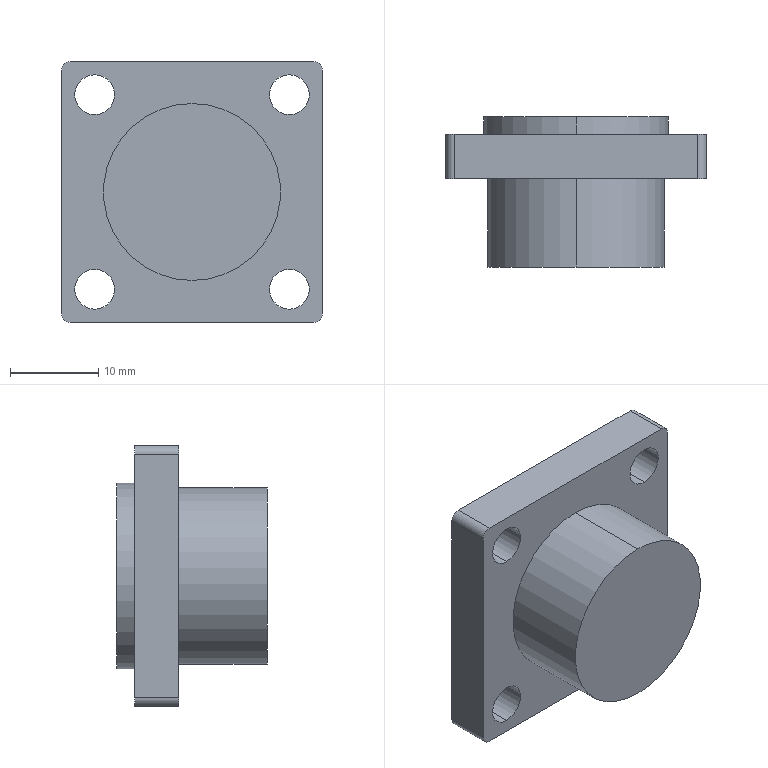Part | SolidWorks | features ICE 5, Extrusion 1, Fillet 1 | 1 solid | 29 faces | box 29.5 x 17 x 29.5 mm | volume 7218 mm3 | cylinder 16 | plane 13 | commonest cylinder face diameters 4.5 x8 2 x4 20 x2 21 x2
STEP:
#1=CARTESIAN_POINT('',(11.,10.,8.75));
#2=VERTEX_POINT('',#1);
#3=CARTESIAN_POINT('',(11.,10.,13.25));
#4=VERTEX_POINT('',#3);
#5=CARTESIAN_POINT('',(11.,10.,11.));
#6=DIRECTION('',(0.,1.,0.));
#7=DIRECTION('',(0.,0.,1.));
#8=AXIS2_PLACEMENT_3D('',#5,#6,#7);
#9=CIRCLE('',#8,2.25);
#10=EDGE_CURVE('',#2,#4,#9,.T.);
#11=ORIENTED_EDGE('',*,*,#10,.F.);
#12=CARTESIAN_POINT('',(11.,15.,8.75));
#13=VERTEX_POINT('',#12);
#14=CARTESIAN_POINT('',(11.,-2.,8.75));
#15=DIRECTION('',(0.,1.,0.));
#16=VECTOR('',#15,1000.);
#17=LINE('',#14,#16);
#18=EDGE_CURVE('',#2,#13,#17,.T.);
#19=ORIENTED_EDGE('',*,*,#18,.T.);
#20=CARTESIAN_POINT('',(11.,15.,13.25));
#21=VERTEX_POINT('',#20);
#22=CARTESIAN_POINT('',(11.,15.,11.));
#23=DIRECTION('',(0.,1.,0.));
#24=DIRECTION('',(0.,0.,1.));
#25=AXIS2_PLACEMENT_3D('',#22,#23,#24);
#26=CIRCLE('',#25,2.25);
#27=EDGE_CURVE('',#13,#21,#26,.T.);
#28=ORIENTED_EDGE('',*,*,#27,.T.);
#29=CARTESIAN_POINT('',(11.,-2.,13.25));
#30=DIRECTION('',(0.,1.,0.));
#31=VECTOR('',#30,1000.);
#32=LINE('',#29,#31);
#33=EDGE_CURVE('',#4,#21,#32,.T.);
#34=ORIENTED_EDGE('',*,*,#33,.F.);
#35=EDGE_LOOP('',(#11,#19,#28,#34));
#36=FACE_OUTER_BOUND('',#35,.T.);
#37=CARTESIAN_POINT('',(11.,-2.,11.));
#38=DIRECTION('',(0.,1.,0.));
#39=DIRECTION('',(0.,0.,1.));
#40=AXIS2_PLACEMENT_3D('',#37,#38,#39);
#41=CYLINDRICAL_SURFACE('',#40,2.25);
#42=ADVANCED_FACE('',(#36),#41,.F.);
#43=CARTESIAN_POINT('',(-11.,10.,8.75));
#44=VERTEX_POINT('',#43);
#45=CARTESIAN_POINT('',(-11.,10.,13.25));
#46=VERTEX_POINT('',#45);
#47=CARTESIAN_POINT('',(-11.,10.,11.));
#48=DIRECTION('',(0.,1.,0.));
#49=DIRECTION('',(0.,0.,1.));
#50=AXIS2_PLACEMENT_3D('',#47,#48,#49);
#51=CIRCLE('',#50,2.25);
#52=EDGE_CURVE('',#44,#46,#51,.T.);
#53=ORIENTED_EDGE('',*,*,#52,.F.);
#54=CARTESIAN_POINT('',(-11.,15.,8.75));
#55=VERTEX_POINT('',#54);
#56=CARTESIAN_POINT('',(-11.,-2.,8.75));
#57=DIRECTION('',(0.,1.,0.));
#58=VECTOR('',#57,1000.);
#59=LINE('',#56,#58);
#60=EDGE_CURVE('',#44,#55,#59,.T.);
#61=ORIENTED_EDGE('',*,*,#60,.T.);
#62=CARTESIAN_POINT('',(-11.,15.,13.25));
#63=VERTEX_POINT('',#62);
#64=CARTESIAN_POINT('',(-11.,15.,11.));
#65=DIRECTION('',(0.,1.,0.));
#66=DIRECTION('',(0.,0.,1.));
#67=AXIS2_PLACEMENT_3D('',#64,#65,#66);
#68=CIRCLE('',#67,2.25);
#69=EDGE_CURVE('',#55,#63,#68,.T.);
#70=ORIENTED_EDGE('',*,*,#69,.T.);
#71=CARTESIAN_POINT('',(-11.,-2.,13.25));
#72=DIRECTION('',(0.,1.,0.));
#73=VECTOR('',#72,1000.);
#74=LINE('',#71,#73);
#75=EDGE_CURVE('',#46,#63,#74,.T.);
#76=ORIENTED_EDGE('',*,*,#75,.F.);
#77=EDGE_LOOP('',(#53,#61,#70,#76));
#78=FACE_OUTER_BOUND('',#77,.T.);
#79=CARTESIAN_POINT('',(-11.,-2.,11.));
#80=DIRECTION('',(0.,1.,0.));
#81=DIRECTION('',(0.,0.,1.));
#82=AXIS2_PLACEMENT_3D('',#79,#80,#81);
#83=CYLINDRICAL_SURFACE('',#82,2.25);
#84=ADVANCED_FACE('',(#78),#83,.F.);
#85=CARTESIAN_POINT('',(-11.,10.,-13.25));
#86=VERTEX_POINT('',#85);
#87=CARTESIAN_POINT('',(-11.,10.,-8.75));
#88=VERTEX_POINT('',#87);
#89=CARTESIAN_POINT('',(-11.,10.,-11.));
#90=DIRECTION('',(0.,1.,0.));
#91=DIRECTION('',(0.,0.,1.));
#92=AXIS2_PLACEMENT_3D('',#89,#90,#91);
#93=CIRCLE('',#92,2.25);
#94=EDGE_CURVE('',#86,#88,#93,.T.);
#95=ORIENTED_EDGE('',*,*,#94,.F.);
#96=CARTESIAN_POINT('',(-11.,15.,-13.25));
#97=VERTEX_POINT('',#96);
#98=CARTESIAN_POINT('',(-11.,-2.,-13.25));
#99=DIRECTION('',(0.,1.,0.));
#100=VECTOR('',#99,1000.);
#101=LINE('',#98,#100);
#102=EDGE_CURVE('',#86,#97,#101,.T.);
#103=ORIENTED_EDGE('',*,*,#102,.T.);
#104=CARTESIAN_POINT('',(-11.,15.,-8.75));
#105=VERTEX_POINT('',#104);
#106=CARTESIAN_POINT('',(-11.,15.,-11.));
#107=DIRECTION('',(0.,1.,0.));
#108=DIRECTION('',(0.,0.,1.));
#109=AXIS2_PLACEMENT_3D('',#106,#107,#108);
#110=CIRCLE('',#109,2.25);
#111=EDGE_CURVE('',#97,#105,#110,.T.);
#112=ORIENTED_EDGE('',*,*,#111,.T.);
#113=CARTESIAN_POINT('',(-11.,-2.,-8.75));
#114=DIRECTION('',(0.,1.,0.));
#115=VECTOR('',#114,1000.);
#116=LINE('',#113,#115);
#117=EDGE_CURVE('',#88,#105,#116,.T.);
#118=ORIENTED_EDGE('',*,*,#117,.F.);
#119=EDGE_LOOP('',(#95,#103,#112,#118));
#120=FACE_OUTER_BOUND('',#119,.T.);
#121=CARTESIAN_POINT('',(-11.,-2.,-11.));
#122=DIRECTION('',(0.,1.,0.));
#123=DIRECTION('',(0.,0.,1.));
#124=AXIS2_PLACEMENT_3D('',#121,#122,#123);
#125=CYLINDRICAL_SURFACE('',#124,2.25);
#126=ADVANCED_FACE('',(#120),#125,.F.);
#127=CARTESIAN_POINT('',(11.,10.,-13.25));
#128=VERTEX_POINT('',#127);
#129=CARTESIAN_POINT('',(11.,10.,-8.75));
#130=VERTEX_POINT('',#129);
#131=CARTESIAN_POINT('',(11.,10.,-11.));
#132=DIRECTION('',(0.,1.,0.));
#133=DIRECTION('',(0.,0.,1.));
#134=AXIS2_PLACEMENT_3D('',#131,#132,#133);
#135=CIRCLE('',#134,2.25);
#136=EDGE_CURVE('',#128,#130,#135,.T.);
#137=ORIENTED_EDGE('',*,*,#136,.F.);
#138=CARTESIAN_POINT('',(11.,15.,-13.25));
#139=VERTEX_POINT('',#138);
#140=CARTESIAN_POINT('',(11.,-2.,-13.25));
#141=DIRECTION('',(0.,1.,0.));
#142=VECTOR('',#141,1000.);
#143=LINE('',#140,#142);
#144=EDGE_CURVE('',#128,#139,#143,.T.);
#145=ORIENTED_EDGE('',*,*,#144,.T.);
#146=CARTESIAN_POINT('',(11.,15.,-8.75));
#147=VERTEX_POINT('',#146);
#148=CARTESIAN_POINT('',(11.,15.,-11.));
#149=DIRECTION('',(0.,1.,0.));
#150=DIRECTION('',(0.,0.,1.));
#151=AXIS2_PLACEMENT_3D('',#148,#149,#150);
#152=CIRCLE('',#151,2.25);
#153=EDGE_CURVE('',#139,#147,#152,.T.);
#154=ORIENTED_EDGE('',*,*,#153,.T.);
#155=CARTESIAN_POINT('',(11.,-2.,-8.75));
#156=DIRECTION('',(0.,1.,0.));
#157=VECTOR('',#156,1000.);
#158=LINE('',#155,#157);
#159=EDGE_CURVE('',#130,#147,#158,.T.);
#160=ORIENTED_EDGE('',*,*,#159,.F.);
#161=EDGE_LOOP('',(#137,#145,#154,#160));
#162=FACE_OUTER_BOUND('',#161,.T.);
#163=CARTESIAN_POINT('',(11.,-2.,-11.));
#164=DIRECTION('',(0.,1.,0.));
#165=DIRECTION('',(0.,0.,1.));
#166=AXIS2_PLACEMENT_3D('',#163,#164,#165);
#167=CYLINDRICAL_SURFACE('',#166,2.25);
#168=ADVANCED_FACE('',(#162),#167,.F.);
#169=CARTESIAN_POINT('',(0.,10.,10.));
#170=VERTEX_POINT('',#169);
#171=CARTESIAN_POINT('',(0.,10.,-10.));
#172=VERTEX_POINT('',#171);
#173=CARTESIAN_POINT('',(0.,10.,0.));
#174=DIRECTION('',(0.,1.,0.));
#175=DIRECTION('',(0.,0.,1.));
#176=AXIS2_PLACEMENT_3D('',#173,#174,#175);
#177=CIRCLE('',#176,10.);
#178=EDGE_CURVE('',#170,#172,#177,.T.);
#179=ORIENTED_EDGE('',*,*,#178,.F.);
#180=CARTESIAN_POINT('',(0.,0.,10.));
#181=VERTEX_POINT('',#180);
#182=CARTESIAN_POINT('',(0.,10.,10.));
#183=DIRECTION('',(0.,-1.,0.));
#184=VECTOR('',#183,1000.);
#185=LINE('',#182,#184);
#186=EDGE_CURVE('',#170,#181,#185,.T.);
#187=ORIENTED_EDGE('',*,*,#186,.T.);
#188=CARTESIAN_POINT('',(0.,0.,-10.));
#189=VERTEX_POINT('',#188);
#190=CARTESIAN_POINT('',(0.,0.,0.));
#191=DIRECTION('',(0.,1.,0.));
#192=DIRECTION('',(0.,0.,1.));
#193=AXIS2_PLACEMENT_3D('',#190,#191,#192);
#194=CIRCLE('',#193,10.);
#195=EDGE_CURVE('',#181,#189,#194,.T.);
#196=ORIENTED_EDGE('',*,*,#195,.T.);
#197=CARTESIAN_POINT('',(0.,10.,-10.));
#198=DIRECTION('',(0.,-1.,0.));
#199=VECTOR('',#198,1000.);
#200=LINE('',#197,#199);
#201=EDGE_CURVE('',#172,#189,#200,.T.);
#202=ORIENTED_EDGE('',*,*,#201,.F.);
#203=EDGE_LOOP('',(#179,#187,#196,#202));
#204=FACE_OUTER_BOUND('',#203,.T.);
#205=CARTESIAN_POINT('',(0.,10.,0.));
#206=DIRECTION('',(0.,-1.,0.));
#207=DIRECTION('',(0.,0.,-1.));
#208=AXIS2_PLACEMENT_3D('',#205,#206,#207);
#209=CYLINDRICAL_SURFACE('',#208,10.);
#210=ADVANCED_FACE('',(#204),#209,.T.);
#211=CARTESIAN_POINT('',(0.,17.,10.5));
#212=VERTEX_POINT('',#211);
#213=CARTESIAN_POINT('',(0.,17.,-10.5));
#214=VERTEX_POINT('',#213);
#215=CARTESIAN_POINT('',(0.,17.,0.));
#216=DIRECTION('',(0.,1.,0.));
#217=DIRECTION('',(0.,0.,1.));
#218=AXIS2_PLACEMENT_3D('',#215,#216,#217);
#219=CIRCLE('',#218,10.5);
#220=EDGE_CURVE('',#212,#214,#219,.T.);
#221=ORIENTED_EDGE('',*,*,#220,.F.);
#222=CARTESIAN_POINT('',(0.,15.,10.5));
#223=VERTEX_POINT('',#222);
#224=CARTESIAN_POINT('',(0.,32.,10.5));
#225=DIRECTION('',(0.,-1.,0.));
#226=VECTOR('',#225,1000.);
#227=LINE('',#224,#226);
#228=EDGE_CURVE('',#212,#223,#227,.T.);
#229=ORIENTED_EDGE('',*,*,#228,.T.);
#230=CARTESIAN_POINT('',(0.,15.,-10.5));
#231=VERTEX_POINT('',#230);
#232=CARTESIAN_POINT('',(0.,15.,0.));
#233=DIRECTION('',(0.,1.,0.));
#234=DIRECTION('',(0.,0.,1.));
#235=AXIS2_PLACEMENT_3D('',#232,#233,#234);
#236=CIRCLE('',#235,10.5);
#237=EDGE_CURVE('',#223,#231,#236,.T.);
#238=ORIENTED_EDGE('',*,*,#237,.T.);
#239=CARTESIAN_POINT('',(0.,32.,-10.5));
#240=DIRECTION('',(0.,-1.,0.));
#241=VECTOR('',#240,1000.);
#242=LINE('',#239,#241);
#243=EDGE_CURVE('',#214,#231,#242,.T.);
#244=ORIENTED_EDGE('',*,*,#243,.F.);
#245=EDGE_LOOP('',(#221,#229,#238,#244));
#246=FACE_OUTER_BOUND('',#245,.T.);
#247=CARTESIAN_POINT('',(0.,32.,0.));
#248=DIRECTION('',(0.,-1.,0.));
#249=DIRECTION('',(0.,0.,-1.));
#250=AXIS2_PLACEMENT_3D('',#247,#248,#249);
#251=CYLINDRICAL_SURFACE('',#250,10.5);
#252=ADVANCED_FACE('',(#246),#251,.T.);
#253=ORIENTED_EDGE('',*,*,#228,.F.);
#254=CARTESIAN_POINT('',(0.,17.,0.));
#255=DIRECTION('',(0.,1.,0.));
#256=DIRECTION('',(0.,0.,1.));
#257=AXIS2_PLACEMENT_3D('',#254,#255,#256);
#258=CIRCLE('',#257,10.5);
#259=EDGE_CURVE('',#214,#212,#258,.T.);
#260=ORIENTED_EDGE('',*,*,#259,.F.);
#261=ORIENTED_EDGE('',*,*,#243,.T.);
#262=CARTESIAN_POINT('',(0.,15.,0.));
#263=DIRECTION('',(0.,1.,0.));
#264=DIRECTION('',(0.,0.,1.));
#265=AXIS2_PLACEMENT_3D('',#262,#263,#264);
#266=CIRCLE('',#265,10.5);
#267=EDGE_CURVE('',#231,#223,#266,.T.);
#268=ORIENTED_EDGE('',*,*,#267,.T.);
#269=EDGE_LOOP('',(#253,#260,#261,#268));
#270=FACE_OUTER_BOUND('',#269,.T.);
#271=CARTESIAN_POINT('',(0.,32.,0.));
#272=DIRECTION('',(0.,-1.,0.));
#273=DIRECTION('',(0.,0.,-1.));
#274=AXIS2_PLACEMENT_3D('',#271,#272,#273);
#275=CYLINDRICAL_SURFACE('',#274,10.5);
#276=ADVANCED_FACE('',(#270),#275,.T.);
#277=CARTESIAN_POINT('',(11.,15.,11.));
#278=DIRECTION('',(0.,1.,0.));
#279=DIRECTION('',(0.,0.,1.));
#280=AXIS2_PLACEMENT_3D('',#277,#278,#279);
#281=CIRCLE('',#280,2.25);
#282=EDGE_CURVE('',#21,#13,#281,.T.);
#283=ORIENTED_EDGE('',*,*,#282,.F.);
#284=ORIENTED_EDGE('',*,*,#27,.F.);
#285=EDGE_LOOP('',(#283,#284));
#286=FACE_BOUND('',#285,.T.);
#287=CARTESIAN_POINT('',(-11.,15.,11.));
#288=DIRECTION('',(0.,1.,0.));
#289=DIRECTION('',(0.,0.,1.));
#290=AXIS2_PLACEMENT_3D('',#287,#288,#289);
#291=CIRCLE('',#290,2.25);
#292=EDGE_CURVE('',#63,#55,#291,.T.);
#293=ORIENTED_EDGE('',*,*,#292,.F.);
#294=ORIENTED_EDGE('',*,*,#69,.F.);
#295=EDGE_LOOP('',(#293,#294));
#296=FACE_BOUND('',#295,.T.);
#297=CARTESIAN_POINT('',(-11.,15.,-11.));
#298=DIRECTION('',(0.,1.,0.));
#299=DIRECTION('',(0.,0.,1.));
#300=AXIS2_PLACEMENT_3D('',#297,#298,#299);
#301=CIRCLE('',#300,2.25);
#302=EDGE_CURVE('',#105,#97,#301,.T.);
#303=ORIENTED_EDGE('',*,*,#302,.F.);
#304=ORIENTED_EDGE('',*,*,#111,.F.);
#305=EDGE_LOOP('',(#303,#304));
#306=FACE_BOUND('',#305,.T.);
#307=CARTESIAN_POINT('',(11.,15.,-11.));
#308=DIRECTION('',(0.,1.,0.));
#309=DIRECTION('',(0.,0.,1.));
#310=AXIS2_PLACEMENT_3D('',#307,#308,#309);
#311=CIRCLE('',#310,2.25);
#312=EDGE_CURVE('',#147,#139,#311,.T.);
#313=ORIENTED_EDGE('',*,*,#312,.F.);
#314=ORIENTED_EDGE('',*,*,#153,.F.);
#315=EDGE_LOOP('',(#313,#314));
#316=FACE_BOUND('',#315,.T.);
#317=CARTESIAN_POINT('',(13.75,15.,-14.75));
#318=VERTEX_POINT('',#317);
#319=CARTESIAN_POINT('',(-13.75,15.,-14.75));
#320=VERTEX_POINT('',#319);
#321=CARTESIAN_POINT('',(-14.75,15.,-14.75));
#322=DIRECTION('',(-1.,0.,0.));
#323=VECTOR('',#322,1000.);
#324=LINE('',#321,#323);
#325=EDGE_CURVE('',#318,#320,#324,.T.);
#326=ORIENTED_EDGE('',*,*,#325,.T.);
#327=CARTESIAN_POINT('',(-14.75,15.,-13.75));
#328=VERTEX_POINT('',#327);
#329=CARTESIAN_POINT('',(-13.75,15.,-13.75));
#330=DIRECTION('',(0.,1.,0.));
#331=DIRECTION('',(0.,0.,1.));
#332=AXIS2_PLACEMENT_3D('',#329,#330,#331);
#333=CIRCLE('',#332,1.);
#334=EDGE_CURVE('',#320,#328,#333,.T.);
#335=ORIENTED_EDGE('',*,*,#334,.T.);
#336=CARTESIAN_POINT('',(-14.75,15.,13.75));
#337=VERTEX_POINT('',#336);
#338=CARTESIAN_POINT('',(-14.75,15.,-14.75));
#339=DIRECTION('',(0.,0.,1.));
#340=VECTOR('',#339,1000.);
#341=LINE('',#338,#340);
#342=EDGE_CURVE('',#328,#337,#341,.T.);
#343=ORIENTED_EDGE('',*,*,#342,.T.);
#344=CARTESIAN_POINT('',(-13.75,15.,14.75));
#345=VERTEX_POINT('',#344);
#346=CARTESIAN_POINT('',(-13.75,15.,13.75));
#347=DIRECTION('',(0.,1.,0.));
#348=DIRECTION('',(0.,0.,1.));
#349=AXIS2_PLACEMENT_3D('',#346,#347,#348);
#350=CIRCLE('',#349,1.);
#351=EDGE_CURVE('',#337,#345,#350,.T.);
#352=ORIENTED_EDGE('',*,*,#351,.T.);
#353=CARTESIAN_POINT('',(13.75,15.,14.75));
#354=VERTEX_POINT('',#353);
#355=CARTESIAN_POINT('',(-14.75,15.,14.75));
#356=DIRECTION('',(1.,0.,0.));
#357=VECTOR('',#356,1000.);
#358=LINE('',#355,#357);
#359=EDGE_CURVE('',#345,#354,#358,.T.);
#360=ORIENTED_EDGE('',*,*,#359,.T.);
#361=CARTESIAN_POINT('',(14.75,15.,13.75));
#362=VERTEX_POINT('',#361);
#363=CARTESIAN_POINT('',(13.75,15.,13.75));
#364=DIRECTION('',(0.,1.,0.));
#365=DIRECTION('',(0.,0.,1.));
#366=AXIS2_PLACEMENT_3D('',#363,#364,#365);
#367=CIRCLE('',#366,1.);
#368=EDGE_CURVE('',#354,#362,#367,.T.);
#369=ORIENTED_EDGE('',*,*,#368,.T.);
#370=CARTESIAN_POINT('',(14.75,15.,-13.75));
#371=VERTEX_POINT('',#370);
#372=CARTESIAN_POINT('',(14.75,15.,-14.75));
#373=DIRECTION('',(0.,0.,-1.));
#374=VECTOR('',#373,1000.);
#375=LINE('',#372,#374);
#376=EDGE_CURVE('',#362,#371,#375,.T.);
#377=ORIENTED_EDGE('',*,*,#376,.T.);
#378=CARTESIAN_POINT('',(13.75,15.,-13.75));
#379=DIRECTION('',(0.,1.,0.));
#380=DIRECTION('',(0.,0.,1.));
#381=AXIS2_PLACEMENT_3D('',#378,#379,#380);
#382=CIRCLE('',#381,1.);
#383=EDGE_CURVE('',#371,#318,#382,.T.);
#384=ORIENTED_EDGE('',*,*,#383,.T.);
#385=EDGE_LOOP('',(#326,#335,#343,#352,#360,#369,#377,#384));
#386=FACE_OUTER_BOUND('',#385,.T.);
#387=ORIENTED_EDGE('',*,*,#267,.F.);
#388=ORIENTED_EDGE('',*,*,#237,.F.);
#389=EDGE_LOOP('',(#387,#388));
#390=FACE_BOUND('',#389,.T.);
#391=CARTESIAN_POINT('',(0.,15.,0.));
#392=DIRECTION('',(0.,1.,0.));
#393=DIRECTION('',(0.,0.,1.));
#394=AXIS2_PLACEMENT_3D('',#391,#392,#393);
#395=PLANE('',#394);
#396=ADVANCED_FACE('',(#286,#296,#306,#316,#386,#390),#395,.T.);
#397=ORIENTED_EDGE('',*,*,#186,.F.);
#398=CARTESIAN_POINT('',(0.,10.,0.));
#399=DIRECTION('',(0.,1.,0.));
#400=DIRECTION('',(0.,0.,1.));
#401=AXIS2_PLACEMENT_3D('',#398,#399,#400);
#402=CIRCLE('',#401,10.);
#403=EDGE_CURVE('',#172,#170,#402,.T.);
#404=ORIENTED_EDGE('',*,*,#403,.F.);
#405=ORIENTED_EDGE('',*,*,#201,.T.);
#406=CARTESIAN_POINT('',(0.,0.,0.));
#407=DIRECTION('',(0.,1.,0.));
#408=DIRECTION('',(0.,0.,1.));
#409=AXIS2_PLACEMENT_3D('',#406,#407,#408);
#410=CIRCLE('',#409,10.);
#411=EDGE_CURVE('',#189,#181,#410,.T.);
#412=ORIENTED_EDGE('',*,*,#411,.T.);
#413=EDGE_LOOP('',(#397,#404,#405,#412));
#414=FACE_OUTER_BOUND('',#413,.T.);
#415=CARTESIAN_POINT('',(0.,10.,0.));
#416=DIRECTION('',(0.,-1.,0.));
#417=DIRECTION('',(0.,0.,-1.));
#418=AXIS2_PLACEMENT_3D('',#415,#416,#417);
#419=CYLINDRICAL_SURFACE('',#418,10.);
#420=ADVANCED_FACE('',(#414),#419,.T.);
#421=ORIENTED_EDGE('',*,*,#411,.F.);
#422=ORIENTED_EDGE('',*,*,#195,.F.);
#423=EDGE_LOOP('',(#421,#422));
#424=FACE_OUTER_BOUND('',#423,.T.);
#425=CARTESIAN_POINT('',(0.,0.,0.));
#426=DIRECTION('',(0.,1.,0.));
#427=DIRECTION('',(0.,0.,1.));
#428=AXIS2_PLACEMENT_3D('',#425,#426,#427);
#429=PLANE('',#428);
#430=ADVANCED_FACE('',(#424),#429,.F.);
#431=CARTESIAN_POINT('',(11.,10.,11.));
#432=DIRECTION('',(0.,1.,0.));
#433=DIRECTION('',(0.,0.,1.));
#434=AXIS2_PLACEMENT_3D('',#431,#432,#433);
#435=CIRCLE('',#434,2.25);
#436=EDGE_CURVE('',#4,#2,#435,.T.);
#437=ORIENTED_EDGE('',*,*,#436,.T.);
#438=ORIENTED_EDGE('',*,*,#10,.T.);
#439=EDGE_LOOP('',(#437,#438));
#440=FACE_BOUND('',#439,.T.);
#441=CARTESIAN_POINT('',(-11.,10.,11.));
#442=DIRECTION('',(0.,1.,0.));
#443=DIRECTION('',(0.,0.,1.));
#444=AXIS2_PLACEMENT_3D('',#441,#442,#443);
#445=CIRCLE('',#444,2.25);
#446=EDGE_CURVE('',#46,#44,#445,.T.);
#447=ORIENTED_EDGE('',*,*,#446,.T.);
#448=ORIENTED_EDGE('',*,*,#52,.T.);
#449=EDGE_LOOP('',(#447,#448));
#450=FACE_BOUND('',#449,.T.);
#451=CARTESIAN_POINT('',(-11.,10.,-11.));
#452=DIRECTION('',(0.,1.,0.));
#453=DIRECTION('',(0.,0.,1.));
#454=AXIS2_PLACEMENT_3D('',#451,#452,#453);
#455=CIRCLE('',#454,2.25);
#456=EDGE_CURVE('',#88,#86,#455,.T.);
#457=ORIENTED_EDGE('',*,*,#456,.T.);
#458=ORIENTED_EDGE('',*,*,#94,.T.);
#459=EDGE_LOOP('',(#457,#458));
#460=FACE_BOUND('',#459,.T.);
#461=CARTESIAN_POINT('',(11.,10.,-11.));
#462=DIRECTION('',(0.,1.,0.));
#463=DIRECTION('',(0.,0.,1.));
#464=AXIS2_PLACEMENT_3D('',#461,#462,#463);
#465=CIRCLE('',#464,2.25);
#466=EDGE_CURVE('',#130,#128,#465,.T.);
#467=ORIENTED_EDGE('',*,*,#466,.T.);
#468=ORIENTED_EDGE('',*,*,#136,.T.);
#469=EDGE_LOOP('',(#467,#468));
#470=FACE_BOUND('',#469,.T.);
#471=CARTESIAN_POINT('',(-14.75,10.,-13.75));
#472=VERTEX_POINT('',#471);
#473=CARTESIAN_POINT('',(-14.75,10.,13.75));
#474=VERTEX_POINT('',#473);
#475=CARTESIAN_POINT('',(-14.75,10.,-14.75));
#476=DIRECTION('',(0.,0.,1.));
#477=VECTOR('',#476,1000.);
#478=LINE('',#475,#477);
#479=EDGE_CURVE('',#472,#474,#478,.T.);
#480=ORIENTED_EDGE('',*,*,#479,.F.);
#481=CARTESIAN_POINT('',(-13.75,10.,-14.75));
#482=VERTEX_POINT('',#481);
#483=CARTESIAN_POINT('',(-13.75,10.,-13.75));
#484=DIRECTION('',(0.,-1.,0.));
#485=DIRECTION('',(0.,0.,1.));
#486=AXIS2_PLACEMENT_3D('',#483,#484,#485);
#487=CIRCLE('',#486,1.);
#488=EDGE_CURVE('',#472,#482,#487,.T.);
#489=ORIENTED_EDGE('',*,*,#488,.T.);
#490=CARTESIAN_POINT('',(13.75,10.,-14.75));
#491=VERTEX_POINT('',#490);
#492=CARTESIAN_POINT('',(-14.75,10.,-14.75));
#493=DIRECTION('',(-1.,0.,0.));
#494=VECTOR('',#493,1000.);
#495=LINE('',#492,#494);
#496=EDGE_CURVE('',#491,#482,#495,.T.);
#497=ORIENTED_EDGE('',*,*,#496,.F.);
#498=CARTESIAN_POINT('',(14.75,10.,-13.75));
#499=VERTEX_POINT('',#498);
#500=CARTESIAN_POINT('',(13.75,10.,-13.75));
#501=DIRECTION('',(0.,-1.,0.));
#502=DIRECTION('',(0.,0.,1.));
#503=AXIS2_PLACEMENT_3D('',#500,#501,#502);
#504=CIRCLE('',#503,1.);
#505=EDGE_CURVE('',#491,#499,#504,.T.);
#506=ORIENTED_EDGE('',*,*,#505,.T.);
#507=CARTESIAN_POINT('',(14.75,10.,13.75));
#508=VERTEX_POINT('',#507);
#509=CARTESIAN_POINT('',(14.75,10.,-14.75));
#510=DIRECTION('',(0.,0.,-1.));
#511=VECTOR('',#510,1000.);
#512=LINE('',#509,#511);
#513=EDGE_CURVE('',#508,#499,#512,.T.);
#514=ORIENTED_EDGE('',*,*,#513,.F.);
#515=CARTESIAN_POINT('',(13.75,10.,14.75));
#516=VERTEX_POINT('',#515);
#517=CARTESIAN_POINT('',(13.75,10.,13.75));
#518=DIRECTION('',(0.,-1.,0.));
#519=DIRECTION('',(0.,0.,1.));
#520=AXIS2_PLACEMENT_3D('',#517,#518,#519);
#521=CIRCLE('',#520,1.);
#522=EDGE_CURVE('',#508,#516,#521,.T.);
#523=ORIENTED_EDGE('',*,*,#522,.T.);
#524=CARTESIAN_POINT('',(-13.75,10.,14.75));
#525=VERTEX_POINT('',#524);
#526=CARTESIAN_POINT('',(-14.75,10.,14.75));
#527=DIRECTION('',(1.,0.,0.));
#528=VECTOR('',#527,1000.);
#529=LINE('',#526,#528);
#530=EDGE_CURVE('',#525,#516,#529,.T.);
#531=ORIENTED_EDGE('',*,*,#530,.F.);
#532=CARTESIAN_POINT('',(-13.75,10.,13.75));
#533=DIRECTION('',(0.,-1.,0.));
#534=DIRECTION('',(0.,0.,1.));
#535=AXIS2_PLACEMENT_3D('',#532,#533,#534);
#536=CIRCLE('',#535,1.);
#537=EDGE_CURVE('',#525,#474,#536,.T.);
#538=ORIENTED_EDGE('',*,*,#537,.T.);
#539=EDGE_LOOP('',(#480,#489,#497,#506,#514,#523,#531,#538));
#540=FACE_OUTER_BOUND('',#539,.T.);
#541=ORIENTED_EDGE('',*,*,#403,.T.);
#542=ORIENTED_EDGE('',*,*,#178,.T.);
#543=EDGE_LOOP('',(#541,#542));
#544=FACE_BOUND('',#543,.T.);
#545=CARTESIAN_POINT('',(0.,10.,0.));
#546=DIRECTION('',(0.,1.,0.));
#547=DIRECTION('',(0.,0.,1.));
#548=AXIS2_PLACEMENT_3D('',#545,#546,#547);
#549=PLANE('',#548);
#550=ADVANCED_FACE('',(#440,#450,#460,#470,#540,#544),#549,.F.);
#551=ORIENTED_EDGE('',*,*,#513,.T.);
#552=CARTESIAN_POINT('',(14.75,15.,-13.75));
#553=DIRECTION('',(0.,1.,0.));
#554=VECTOR('',#553,1000.);
#555=LINE('',#552,#554);
#556=EDGE_CURVE('',#499,#371,#555,.T.);
#557=ORIENTED_EDGE('',*,*,#556,.T.);
#558=ORIENTED_EDGE('',*,*,#376,.F.);
#559=CARTESIAN_POINT('',(14.75,15.,13.75));
#560=DIRECTION('',(0.,-1.,0.));
#561=VECTOR('',#560,1000.);
#562=LINE('',#559,#561);
#563=EDGE_CURVE('',#362,#508,#562,.T.);
#564=ORIENTED_EDGE('',*,*,#563,.T.);
#565=EDGE_LOOP('',(#551,#557,#558,#564));
#566=FACE_OUTER_BOUND('',#565,.T.);
#567=CARTESIAN_POINT('',(14.75,15.,-14.75));
#568=DIRECTION('',(-1.,0.,0.));
#569=DIRECTION('',(0.,0.,1.));
#570=AXIS2_PLACEMENT_3D('',#567,#568,#569);
#571=PLANE('',#570);
#572=ADVANCED_FACE('',(#566),#571,.F.);
#573=ORIENTED_EDGE('',*,*,#496,.T.);
#574=CARTESIAN_POINT('',(-13.75,15.,-14.75));
#575=DIRECTION('',(0.,1.,0.));
#576=VECTOR('',#575,1000.);
#577=LINE('',#574,#576);
#578=EDGE_CURVE('',#482,#320,#577,.T.);
#579=ORIENTED_EDGE('',*,*,#578,.T.);
#580=ORIENTED_EDGE('',*,*,#325,.F.);
#581=CARTESIAN_POINT('',(13.75,15.,-14.75));
#582=DIRECTION('',(0.,-1.,0.));
#583=VECTOR('',#582,1000.);
#584=LINE('',#581,#583);
#585=EDGE_CURVE('',#318,#491,#584,.T.);
#586=ORIENTED_EDGE('',*,*,#585,.T.);
#587=EDGE_LOOP('',(#573,#579,#580,#586));
#588=FACE_OUTER_BOUND('',#587,.T.);
#589=CARTESIAN_POINT('',(-14.75,15.,-14.75));
#590=DIRECTION('',(0.,0.,1.));
#591=DIRECTION('',(1.,0.,0.));
#592=AXIS2_PLACEMENT_3D('',#589,#590,#591);
#593=PLANE('',#592);
#594=ADVANCED_FACE('',(#588),#593,.F.);
#595=ORIENTED_EDGE('',*,*,#342,.F.);
#596=CARTESIAN_POINT('',(-14.75,15.,-13.75));
#597=DIRECTION('',(0.,-1.,0.));
#598=VECTOR('',#597,1000.);
#599=LINE('',#596,#598);
#600=EDGE_CURVE('',#328,#472,#599,.T.);
#601=ORIENTED_EDGE('',*,*,#600,.T.);
#602=ORIENTED_EDGE('',*,*,#479,.T.);
#603=CARTESIAN_POINT('',(-14.75,15.,13.75));
#604=DIRECTION('',(0.,1.,0.));
#605=VECTOR('',#604,1000.);
#606=LINE('',#603,#605);
#607=EDGE_CURVE('',#474,#337,#606,.T.);
#608=ORIENTED_EDGE('',*,*,#607,.T.);
#609=EDGE_LOOP('',(#595,#601,#602,#608));
#610=FACE_OUTER_BOUND('',#609,.T.);
#611=CARTESIAN_POINT('',(-14.75,15.,-14.75));
#612=DIRECTION('',(1.,0.,0.));
#613=DIRECTION('',(0.,0.,-1.));
#614=AXIS2_PLACEMENT_3D('',#611,#612,#613);
#615=PLANE('',#614);
#616=ADVANCED_FACE('',(#610),#615,.F.);
#617=ORIENTED_EDGE('',*,*,#530,.T.);
#618=CARTESIAN_POINT('',(13.75,15.,14.75));
#619=DIRECTION('',(0.,1.,0.));
#620=VECTOR('',#619,1000.);
#621=LINE('',#618,#620);
#622=EDGE_CURVE('',#516,#354,#621,.T.);
#623=ORIENTED_EDGE('',*,*,#622,.T.);
#624=ORIENTED_EDGE('',*,*,#359,.F.);
#625=CARTESIAN_POINT('',(-13.75,15.,14.75));
#626=DIRECTION('',(0.,-1.,0.));
#627=VECTOR('',#626,1000.);
#628=LINE('',#625,#627);
#629=EDGE_CURVE('',#345,#525,#628,.T.);
#630=ORIENTED_EDGE('',*,*,#629,.T.);
#631=EDGE_LOOP('',(#617,#623,#624,#630));
#632=FACE_OUTER_BOUND('',#631,.T.);
#633=CARTESIAN_POINT('',(-14.75,15.,14.75));
#634=DIRECTION('',(0.,0.,-1.));
#635=DIRECTION('',(-1.,0.,0.));
#636=AXIS2_PLACEMENT_3D('',#633,#634,#635);
#637=PLANE('',#636);
#638=ADVANCED_FACE('',(#632),#637,.F.);
#639=ORIENTED_EDGE('',*,*,#144,.F.);
#640=ORIENTED_EDGE('',*,*,#466,.F.);
#641=ORIENTED_EDGE('',*,*,#159,.T.);
#642=ORIENTED_EDGE('',*,*,#312,.T.);
#643=EDGE_LOOP('',(#639,#640,#641,#642));
#644=FACE_OUTER_BOUND('',#643,.T.);
#645=CARTESIAN_POINT('',(11.,-2.,-11.));
#646=DIRECTION('',(0.,1.,0.));
#647=DIRECTION('',(0.,0.,1.));
#648=AXIS2_PLACEMENT_3D('',#645,#646,#647);
#649=CYLINDRICAL_SURFACE('',#648,2.25);
#650=ADVANCED_FACE('',(#644),#649,.F.);
#651=ORIENTED_EDGE('',*,*,#102,.F.);
#652=ORIENTED_EDGE('',*,*,#456,.F.);
#653=ORIENTED_EDGE('',*,*,#117,.T.);
#654=ORIENTED_EDGE('',*,*,#302,.T.);
#655=EDGE_LOOP('',(#651,#652,#653,#654));
#656=FACE_OUTER_BOUND('',#655,.T.);
#657=CARTESIAN_POINT('',(-11.,-2.,-11.));
#658=DIRECTION('',(0.,1.,0.));
#659=DIRECTION('',(0.,0.,1.));
#660=AXIS2_PLACEMENT_3D('',#657,#658,#659);
#661=CYLINDRICAL_SURFACE('',#660,2.25);
#662=ADVANCED_FACE('',(#656),#661,.F.);
#663=ORIENTED_EDGE('',*,*,#60,.F.);
#664=ORIENTED_EDGE('',*,*,#446,.F.);
#665=ORIENTED_EDGE('',*,*,#75,.T.);
#666=ORIENTED_EDGE('',*,*,#292,.T.);
#667=EDGE_LOOP('',(#663,#664,#665,#666));
#668=FACE_OUTER_BOUND('',#667,.T.);
#669=CARTESIAN_POINT('',(-11.,-2.,11.));
#670=DIRECTION('',(0.,1.,0.));
#671=DIRECTION('',(0.,0.,1.));
#672=AXIS2_PLACEMENT_3D('',#669,#670,#671);
#673=CYLINDRICAL_SURFACE('',#672,2.25);
#674=ADVANCED_FACE('',(#668),#673,.F.);
#675=ORIENTED_EDGE('',*,*,#18,.F.);
#676=ORIENTED_EDGE('',*,*,#436,.F.);
#677=ORIENTED_EDGE('',*,*,#33,.T.);
#678=ORIENTED_EDGE('',*,*,#282,.T.);
#679=EDGE_LOOP('',(#675,#676,#677,#678));
#680=FACE_OUTER_BOUND('',#679,.T.);
#681=CARTESIAN_POINT('',(11.,-2.,11.));
#682=DIRECTION('',(0.,1.,0.));
#683=DIRECTION('',(0.,0.,1.));
#684=AXIS2_PLACEMENT_3D('',#681,#682,#683);
#685=CYLINDRICAL_SURFACE('',#684,2.25);
#686=ADVANCED_FACE('',(#680),#685,.F.);
#687=ORIENTED_EDGE('',*,*,#334,.F.);
#688=ORIENTED_EDGE('',*,*,#578,.F.);
#689=ORIENTED_EDGE('',*,*,#488,.F.);
#690=ORIENTED_EDGE('',*,*,#600,.F.);
#691=EDGE_LOOP('',(#687,#688,#689,#690));
#692=FACE_OUTER_BOUND('',#691,.T.);
#693=CARTESIAN_POINT('',(-13.75,15.,-13.75));
#694=DIRECTION('',(0.,-1.,0.));
#695=DIRECTION('',(0.,0.,-1.));
#696=AXIS2_PLACEMENT_3D('',#693,#694,#695);
#697=CYLINDRICAL_SURFACE('',#696,1.);
#698=ADVANCED_FACE('',(#692),#697,.T.);
#699=ORIENTED_EDGE('',*,*,#383,.F.);
#700=ORIENTED_EDGE('',*,*,#556,.F.);
#701=ORIENTED_EDGE('',*,*,#505,.F.);
#702=ORIENTED_EDGE('',*,*,#585,.F.);
#703=EDGE_LOOP('',(#699,#700,#701,#702));
#704=FACE_OUTER_BOUND('',#703,.T.);
#705=CARTESIAN_POINT('',(13.75,15.,-13.75));
#706=DIRECTION('',(0.,-1.,0.));
#707=DIRECTION('',(0.,0.,-1.));
#708=AXIS2_PLACEMENT_3D('',#705,#706,#707);
#709=CYLINDRICAL_SURFACE('',#708,1.);
#710=ADVANCED_FACE('',(#704),#709,.T.);
#711=ORIENTED_EDGE('',*,*,#368,.F.);
#712=ORIENTED_EDGE('',*,*,#622,.F.);
#713=ORIENTED_EDGE('',*,*,#522,.F.);
#714=ORIENTED_EDGE('',*,*,#563,.F.);
#715=EDGE_LOOP('',(#711,#712,#713,#714));
#716=FACE_OUTER_BOUND('',#715,.T.);
#717=CARTESIAN_POINT('',(13.75,15.,13.75));
#718=DIRECTION('',(0.,-1.,0.));
#719=DIRECTION('',(0.,0.,-1.));
#720=AXIS2_PLACEMENT_3D('',#717,#718,#719);
#721=CYLINDRICAL_SURFACE('',#720,1.);
#722=ADVANCED_FACE('',(#716),#721,.T.);
#723=ORIENTED_EDGE('',*,*,#351,.F.);
#724=ORIENTED_EDGE('',*,*,#607,.F.);
#725=ORIENTED_EDGE('',*,*,#537,.F.);
#726=ORIENTED_EDGE('',*,*,#629,.F.);
#727=EDGE_LOOP('',(#723,#724,#725,#726));
#728=FACE_OUTER_BOUND('',#727,.T.);
#729=CARTESIAN_POINT('',(-13.75,15.,13.75));
#730=DIRECTION('',(0.,-1.,0.));
#731=DIRECTION('',(0.,0.,-1.));
#732=AXIS2_PLACEMENT_3D('',#729,#730,#731);
#733=CYLINDRICAL_SURFACE('',#732,1.);
#734=ADVANCED_FACE('',(#728),#733,.T.);
#735=CARTESIAN_POINT('',(5.287,17.,6.101));
#736=VERTEX_POINT('',#735);
#737=CARTESIAN_POINT('',(5.287,17.,-6.101));
#738=VERTEX_POINT('',#737);
#739=CARTESIAN_POINT('',(5.287,17.,-6.101));
#740=DIRECTION('',(0.,0.,-1.));
#741=VECTOR('',#740,1000.);
#742=LINE('',#739,#741);
#743=EDGE_CURVE('',#736,#738,#742,.T.);
#744=ORIENTED_EDGE('',*,*,#743,.F.);
#745=CARTESIAN_POINT('',(-5.287,17.,6.101));
#746=VERTEX_POINT('',#745);
#747=CARTESIAN_POINT('',(-5.287,17.,6.101));
#748=DIRECTION('',(1.,0.,0.));
#749=VECTOR('',#748,1000.);
#750=LINE('',#747,#749);
#751=EDGE_CURVE('',#746,#736,#750,.T.);
#752=ORIENTED_EDGE('',*,*,#751,.F.);
#753=CARTESIAN_POINT('',(-5.287,17.,-6.101));
#754=VERTEX_POINT('',#753);
#755=CARTESIAN_POINT('',(-5.287,17.,-6.101));
#756=DIRECTION('',(0.,0.,1.));
#757=VECTOR('',#756,1000.);
#758=LINE('',#755,#757);
#759=EDGE_CURVE('',#754,#746,#758,.T.);
#760=ORIENTED_EDGE('',*,*,#759,.F.);
#761=CARTESIAN_POINT('',(-5.287,17.,-6.101));
#762=DIRECTION('',(-1.,0.,0.));
#763=VECTOR('',#762,1000.);
#764=LINE('',#761,#763);
#765=EDGE_CURVE('',#738,#754,#764,.T.);
#766=ORIENTED_EDGE('',*,*,#765,.F.);
#767=EDGE_LOOP('',(#744,#752,#760,#766));
#768=FACE_BOUND('',#767,.T.);
#769=ORIENTED_EDGE('',*,*,#259,.T.);
#770=ORIENTED_EDGE('',*,*,#220,.T.);
#771=EDGE_LOOP('',(#769,#770));
#772=FACE_OUTER_BOUND('',#771,.T.);
#773=CARTESIAN_POINT('',(0.,17.,0.));
#774=DIRECTION('',(0.,1.,0.));
#775=DIRECTION('',(0.,0.,1.));
#776=AXIS2_PLACEMENT_3D('',#773,#774,#775);
#777=PLANE('',#776);
#778=ADVANCED_FACE('',(#768,#772),#777,.T.);
#779=ORIENTED_EDGE('',*,*,#743,.T.);
#780=CARTESIAN_POINT('',(5.287,12.,-6.101));
#781=VERTEX_POINT('',#780);
#782=CARTESIAN_POINT('',(5.287,12.,-6.101));
#783=DIRECTION('',(0.,1.,0.));
#784=VECTOR('',#783,1000.);
#785=LINE('',#782,#784);
#786=EDGE_CURVE('',#781,#738,#785,.T.);
#787=ORIENTED_EDGE('',*,*,#786,.F.);
#788=CARTESIAN_POINT('',(5.287,12.,6.101));
#789=VERTEX_POINT('',#788);
#790=CARTESIAN_POINT('',(5.287,12.,-6.101));
#791=DIRECTION('',(0.,0.,-1.));
#792=VECTOR('',#791,1000.);
#793=LINE('',#790,#792);
#794=EDGE_CURVE('',#789,#781,#793,.T.);
#795=ORIENTED_EDGE('',*,*,#794,.F.);
#796=CARTESIAN_POINT('',(5.287,12.,6.101));
#797=DIRECTION('',(0.,1.,0.));
#798=VECTOR('',#797,1000.);
#799=LINE('',#796,#798);
#800=EDGE_CURVE('',#789,#736,#799,.T.);
#801=ORIENTED_EDGE('',*,*,#800,.T.);
#802=EDGE_LOOP('',(#779,#787,#795,#801));
#803=FACE_OUTER_BOUND('',#802,.T.);
#804=CARTESIAN_POINT('',(5.287,12.,-6.101));
#805=DIRECTION('',(1.,0.,0.));
#806=DIRECTION('',(0.,0.,-1.));
#807=AXIS2_PLACEMENT_3D('',#804,#805,#806);
#808=PLANE('',#807);
#809=ADVANCED_FACE('',(#803),#808,.F.);
#810=ORIENTED_EDGE('',*,*,#751,.T.);
#811=ORIENTED_EDGE('',*,*,#800,.F.);
#812=CARTESIAN_POINT('',(-5.287,12.,6.101));
#813=VERTEX_POINT('',#812);
#814=CARTESIAN_POINT('',(-5.287,12.,6.101));
#815=DIRECTION('',(1.,0.,0.));
#816=VECTOR('',#815,1000.);
#817=LINE('',#814,#816);
#818=EDGE_CURVE('',#813,#789,#817,.T.);
#819=ORIENTED_EDGE('',*,*,#818,.F.);
#820=CARTESIAN_POINT('',(-5.287,12.,6.101));
#821=DIRECTION('',(0.,1.,0.));
#822=VECTOR('',#821,1000.);
#823=LINE('',#820,#822);
#824=EDGE_CURVE('',#813,#746,#823,.T.);
#825=ORIENTED_EDGE('',*,*,#824,.T.);
#826=EDGE_LOOP('',(#810,#811,#819,#825));
#827=FACE_OUTER_BOUND('',#826,.T.);
#828=CARTESIAN_POINT('',(-5.287,12.,6.101));
#829=DIRECTION('',(0.,0.,1.));
#830=DIRECTION('',(1.,0.,0.));
#831=AXIS2_PLACEMENT_3D('',#828,#829,#830);
#832=PLANE('',#831);
#833=ADVANCED_FACE('',(#827),#832,.F.);
#834=ORIENTED_EDGE('',*,*,#759,.T.);
#835=ORIENTED_EDGE('',*,*,#824,.F.);
#836=CARTESIAN_POINT('',(-5.287,12.,-6.101));
#837=VERTEX_POINT('',#836);
#838=CARTESIAN_POINT('',(-5.287,12.,-6.101));
#839=DIRECTION('',(0.,0.,1.));
#840=VECTOR('',#839,1000.);
#841=LINE('',#838,#840);
#842=EDGE_CURVE('',#837,#813,#841,.T.);
#843=ORIENTED_EDGE('',*,*,#842,.F.);
#844=CARTESIAN_POINT('',(-5.287,12.,-6.101));
#845=DIRECTION('',(0.,1.,0.));
#846=VECTOR('',#845,1000.);
#847=LINE('',#844,#846);
#848=EDGE_CURVE('',#837,#754,#847,.T.);
#849=ORIENTED_EDGE('',*,*,#848,.T.);
#850=EDGE_LOOP('',(#834,#835,#843,#849));
#851=FACE_OUTER_BOUND('',#850,.T.);
#852=CARTESIAN_POINT('',(-5.287,12.,-6.101));
#853=DIRECTION('',(-1.,0.,0.));
#854=DIRECTION('',(0.,0.,1.));
#855=AXIS2_PLACEMENT_3D('',#852,#853,#854);
#856=PLANE('',#855);
#857=ADVANCED_FACE('',(#851),#856,.F.);
#858=ORIENTED_EDGE('',*,*,#765,.T.);
#859=ORIENTED_EDGE('',*,*,#848,.F.);
#860=CARTESIAN_POINT('',(-5.287,12.,-6.101));
#861=DIRECTION('',(-1.,0.,0.));
#862=VECTOR('',#861,1000.);
#863=LINE('',#860,#862);
#864=EDGE_CURVE('',#781,#837,#863,.T.);
#865=ORIENTED_EDGE('',*,*,#864,.F.);
#866=ORIENTED_EDGE('',*,*,#786,.T.);
#867=EDGE_LOOP('',(#858,#859,#865,#866));
#868=FACE_OUTER_BOUND('',#867,.T.);
#869=CARTESIAN_POINT('',(-5.287,12.,-6.101));
#870=DIRECTION('',(0.,0.,-1.));
#871=DIRECTION('',(-1.,0.,0.));
#872=AXIS2_PLACEMENT_3D('',#869,#870,#871);
#873=PLANE('',#872);
#874=ADVANCED_FACE('',(#868),#873,.F.);
#875=ORIENTED_EDGE('',*,*,#794,.T.);
#876=ORIENTED_EDGE('',*,*,#864,.T.);
#877=ORIENTED_EDGE('',*,*,#842,.T.);
#878=ORIENTED_EDGE('',*,*,#818,.T.);
#879=EDGE_LOOP('',(#875,#876,#877,#878));
#880=FACE_OUTER_BOUND('',#879,.T.);
#881=CARTESIAN_POINT('',(0.,12.,0.));
#882=DIRECTION('',(0.,1.,0.));
#883=DIRECTION('',(0.,0.,1.));
#884=AXIS2_PLACEMENT_3D('',#881,#882,#883);
#885=PLANE('',#884);
#886=ADVANCED_FACE('',(#880),#885,.T.);
#887=CLOSED_SHELL('',(#42,#84,#126,#168,#210,#252,#276,#396,#420,#430,#550,#572,#594,#616,#638,#650,#662,#674,#686,#698,#710,#722,#734,#778,#809,#833,#857,#874,#886));
#888=MANIFOLD_SOLID_BREP('',#887);
#889=CARTESIAN_POINT('',(0.,0.,0.));
#890=DIRECTION('',(0.,0.,1.));
#891=DIRECTION('',(1.,0.,0.));
#892=AXIS2_PLACEMENT_3D('',#889,#890,#891);
#893=(LENGTH_UNIT()NAMED_UNIT(*)SI_UNIT(.MILLI.,.METRE.));
#894=UNCERTAINTY_MEASURE_WITH_UNIT(LENGTH_MEASURE(0.00001),#893,'','');
#895=(NAMED_UNIT(*)PLANE_ANGLE_UNIT()SI_UNIT($,.RADIAN.));
#896=(NAMED_UNIT(*)SI_UNIT($,.STERADIAN.)SOLID_ANGLE_UNIT());
#897=(GEOMETRIC_REPRESENTATION_CONTEXT(3)GLOBAL_UNCERTAINTY_ASSIGNED_CONTEXT((#894))GLOBAL_UNIT_ASSIGNED_CONTEXT((#893,#895,#896))REPRESENTATION_CONTEXT('',''));
#898=ADVANCED_BREP_SHAPE_REPRESENTATION('',(#888,#892),#897);